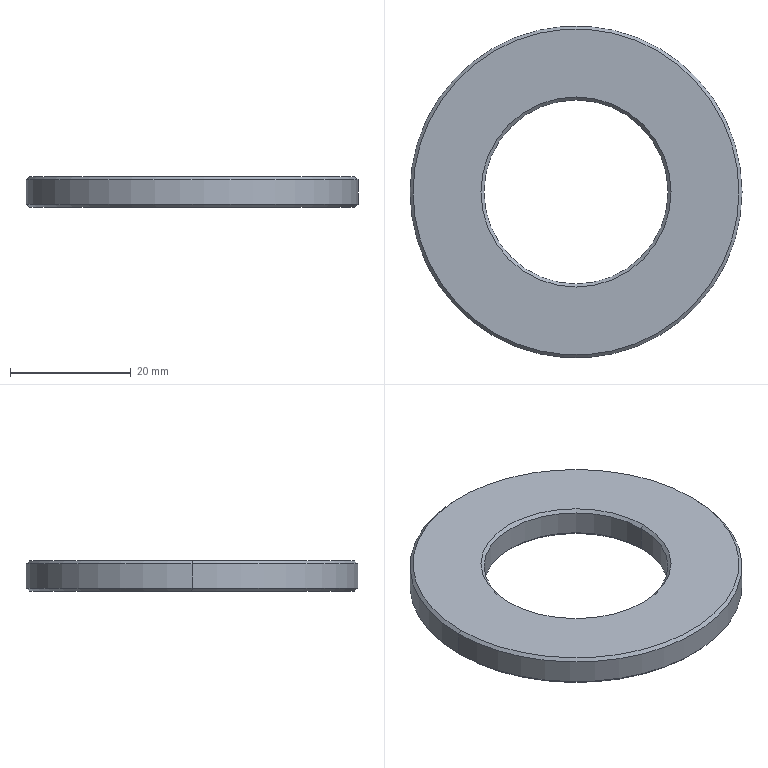Part | STEP file | PN_0001-01-08 Pad | 1 solid | 14 faces | box 55 x 55 x 5 mm | volume 8159 mm3 | cone 8 | cylinder 4 | plane 2 | commonest cylinder face diameters 30.5 x2 55 x2
STEP:
#1=CARTESIAN_POINT('',(27.,0.,5.));
#2=VERTEX_POINT('',#1);
#3=CARTESIAN_POINT('',(-27.,0.,5.));
#4=VERTEX_POINT('',#3);
#5=CARTESIAN_POINT('',(0.,0.,5.));
#6=DIRECTION('',(0.,0.,1.));
#7=DIRECTION('',(1.,0.,0.));
#8=AXIS2_PLACEMENT_3D('',#5,#6,#7);
#9=CIRCLE('',#8,27.);
#10=EDGE_CURVE('',#2,#4,#9,.T.);
#11=ORIENTED_EDGE('',*,*,#10,.F.);
#12=CARTESIAN_POINT('',(27.5,0.,4.5));
#13=VERTEX_POINT('',#12);
#14=CARTESIAN_POINT('',(27.,0.,5.));
#15=DIRECTION('',(0.7071,0.,-0.7071));
#16=VECTOR('',#15,1000.);
#17=LINE('',#14,#16);
#18=EDGE_CURVE('',#2,#13,#17,.T.);
#19=ORIENTED_EDGE('',*,*,#18,.T.);
#20=CARTESIAN_POINT('',(-27.5,0.,4.5));
#21=VERTEX_POINT('',#20);
#22=CARTESIAN_POINT('',(0.,0.,4.5));
#23=DIRECTION('',(0.,0.,-1.));
#24=DIRECTION('',(1.,0.,0.));
#25=AXIS2_PLACEMENT_3D('',#22,#23,#24);
#26=CIRCLE('',#25,27.5);
#27=EDGE_CURVE('',#21,#13,#26,.T.);
#28=ORIENTED_EDGE('',*,*,#27,.F.);
#29=CARTESIAN_POINT('',(-27.,0.,5.));
#30=DIRECTION('',(-0.7071,0.,-0.7071));
#31=VECTOR('',#30,1000.);
#32=LINE('',#29,#31);
#33=EDGE_CURVE('',#4,#21,#32,.T.);
#34=ORIENTED_EDGE('',*,*,#33,.F.);
#35=EDGE_LOOP('',(#11,#19,#28,#34));
#36=FACE_OUTER_BOUND('',#35,.T.);
#37=CARTESIAN_POINT('',(0.,0.,5.));
#38=DIRECTION('',(0.,0.,-1.));
#39=DIRECTION('',(-1.,0.,0.));
#40=AXIS2_PLACEMENT_3D('',#37,#38,#39);
#41=CONICAL_SURFACE('',#40,27.,0.7854);
#42=ADVANCED_FACE('',(#36),#41,.T.);
#43=CARTESIAN_POINT('',(-27.,0.,0.));
#44=VERTEX_POINT('',#43);
#45=CARTESIAN_POINT('',(27.,0.,0.));
#46=VERTEX_POINT('',#45);
#47=CARTESIAN_POINT('',(0.,0.,0.));
#48=DIRECTION('',(0.,0.,-1.));
#49=DIRECTION('',(1.,0.,0.));
#50=AXIS2_PLACEMENT_3D('',#47,#48,#49);
#51=CIRCLE('',#50,27.);
#52=EDGE_CURVE('',#44,#46,#51,.T.);
#53=ORIENTED_EDGE('',*,*,#52,.F.);
#54=CARTESIAN_POINT('',(-27.5,0.,0.5));
#55=VERTEX_POINT('',#54);
#56=CARTESIAN_POINT('',(-27.5,0.,0.5));
#57=DIRECTION('',(-0.7071,0.,0.7071));
#58=VECTOR('',#57,1000.);
#59=LINE('',#56,#58);
#60=EDGE_CURVE('',#44,#55,#59,.T.);
#61=ORIENTED_EDGE('',*,*,#60,.T.);
#62=CARTESIAN_POINT('',(27.5,0.,0.5));
#63=VERTEX_POINT('',#62);
#64=CARTESIAN_POINT('',(0.,0.,0.5));
#65=DIRECTION('',(0.,0.,1.));
#66=DIRECTION('',(1.,0.,0.));
#67=AXIS2_PLACEMENT_3D('',#64,#65,#66);
#68=CIRCLE('',#67,27.5);
#69=EDGE_CURVE('',#63,#55,#68,.T.);
#70=ORIENTED_EDGE('',*,*,#69,.F.);
#71=CARTESIAN_POINT('',(27.5,0.,0.5));
#72=DIRECTION('',(0.7071,0.,0.7071));
#73=VECTOR('',#72,1000.);
#74=LINE('',#71,#73);
#75=EDGE_CURVE('',#46,#63,#74,.T.);
#76=ORIENTED_EDGE('',*,*,#75,.F.);
#77=EDGE_LOOP('',(#53,#61,#70,#76));
#78=FACE_OUTER_BOUND('',#77,.T.);
#79=CARTESIAN_POINT('',(0.,0.,0.5));
#80=DIRECTION('',(0.,0.,1.));
#81=DIRECTION('',(1.,0.,0.));
#82=AXIS2_PLACEMENT_3D('',#79,#80,#81);
#83=CONICAL_SURFACE('',#82,27.5,0.7854);
#84=ADVANCED_FACE('',(#78),#83,.T.);
#85=CARTESIAN_POINT('',(-15.25,0.,4.5));
#86=VERTEX_POINT('',#85);
#87=CARTESIAN_POINT('',(15.25,0.,4.5));
#88=VERTEX_POINT('',#87);
#89=CARTESIAN_POINT('',(0.,0.,4.5));
#90=DIRECTION('',(0.,0.,1.));
#91=DIRECTION('',(1.,0.,0.));
#92=AXIS2_PLACEMENT_3D('',#89,#90,#91);
#93=CIRCLE('',#92,15.25);
#94=EDGE_CURVE('',#86,#88,#93,.T.);
#95=ORIENTED_EDGE('',*,*,#94,.F.);
#96=CARTESIAN_POINT('',(-15.75,0.,5.));
#97=VERTEX_POINT('',#96);
#98=CARTESIAN_POINT('',(-15.25,0.,4.5));
#99=DIRECTION('',(-0.7071,0.,0.7071));
#100=VECTOR('',#99,1000.);
#101=LINE('',#98,#100);
#102=EDGE_CURVE('',#86,#97,#101,.T.);
#103=ORIENTED_EDGE('',*,*,#102,.T.);
#104=CARTESIAN_POINT('',(15.75,0.,5.));
#105=VERTEX_POINT('',#104);
#106=CARTESIAN_POINT('',(0.,0.,5.));
#107=DIRECTION('',(0.,0.,-1.));
#108=DIRECTION('',(1.,0.,0.));
#109=AXIS2_PLACEMENT_3D('',#106,#107,#108);
#110=CIRCLE('',#109,15.75);
#111=EDGE_CURVE('',#105,#97,#110,.T.);
#112=ORIENTED_EDGE('',*,*,#111,.F.);
#113=CARTESIAN_POINT('',(15.25,0.,4.5));
#114=DIRECTION('',(0.7071,0.,0.7071));
#115=VECTOR('',#114,1000.);
#116=LINE('',#113,#115);
#117=EDGE_CURVE('',#88,#105,#116,.T.);
#118=ORIENTED_EDGE('',*,*,#117,.F.);
#119=EDGE_LOOP('',(#95,#103,#112,#118));
#120=FACE_OUTER_BOUND('',#119,.T.);
#121=CARTESIAN_POINT('',(0.,0.,4.5));
#122=DIRECTION('',(0.,0.,1.));
#123=DIRECTION('',(1.,0.,0.));
#124=AXIS2_PLACEMENT_3D('',#121,#122,#123);
#125=CONICAL_SURFACE('',#124,15.25,0.7854);
#126=ADVANCED_FACE('',(#120),#125,.F.);
#127=CARTESIAN_POINT('',(15.25,0.,0.5));
#128=VERTEX_POINT('',#127);
#129=CARTESIAN_POINT('',(-15.25,0.,0.5));
#130=VERTEX_POINT('',#129);
#131=CARTESIAN_POINT('',(0.,0.,0.5));
#132=DIRECTION('',(0.,0.,-1.));
#133=DIRECTION('',(1.,0.,0.));
#134=AXIS2_PLACEMENT_3D('',#131,#132,#133);
#135=CIRCLE('',#134,15.25);
#136=EDGE_CURVE('',#128,#130,#135,.T.);
#137=ORIENTED_EDGE('',*,*,#136,.F.);
#138=CARTESIAN_POINT('',(15.75,0.,0.));
#139=VERTEX_POINT('',#138);
#140=CARTESIAN_POINT('',(15.75,0.,0.));
#141=DIRECTION('',(0.7071,0.,-0.7071));
#142=VECTOR('',#141,1000.);
#143=LINE('',#140,#142);
#144=EDGE_CURVE('',#128,#139,#143,.T.);
#145=ORIENTED_EDGE('',*,*,#144,.T.);
#146=CARTESIAN_POINT('',(-15.75,0.,0.));
#147=VERTEX_POINT('',#146);
#148=CARTESIAN_POINT('',(0.,0.,0.));
#149=DIRECTION('',(0.,0.,1.));
#150=DIRECTION('',(1.,0.,0.));
#151=AXIS2_PLACEMENT_3D('',#148,#149,#150);
#152=CIRCLE('',#151,15.75);
#153=EDGE_CURVE('',#147,#139,#152,.T.);
#154=ORIENTED_EDGE('',*,*,#153,.F.);
#155=CARTESIAN_POINT('',(-15.75,0.,0.));
#156=DIRECTION('',(-0.7071,0.,-0.7071));
#157=VECTOR('',#156,1000.);
#158=LINE('',#155,#157);
#159=EDGE_CURVE('',#130,#147,#158,.T.);
#160=ORIENTED_EDGE('',*,*,#159,.F.);
#161=EDGE_LOOP('',(#137,#145,#154,#160));
#162=FACE_OUTER_BOUND('',#161,.T.);
#163=CARTESIAN_POINT('',(0.,0.,0.));
#164=DIRECTION('',(0.,0.,-1.));
#165=DIRECTION('',(-1.,0.,0.));
#166=AXIS2_PLACEMENT_3D('',#163,#164,#165);
#167=CONICAL_SURFACE('',#166,15.75,0.7854);
#168=ADVANCED_FACE('',(#162),#167,.F.);
#169=ORIENTED_EDGE('',*,*,#94,.T.);
#170=CARTESIAN_POINT('',(15.25,0.,5.));
#171=DIRECTION('',(0.,0.,-1.));
#172=VECTOR('',#171,1000.);
#173=LINE('',#170,#172);
#174=EDGE_CURVE('',#88,#128,#173,.T.);
#175=ORIENTED_EDGE('',*,*,#174,.T.);
#176=ORIENTED_EDGE('',*,*,#136,.T.);
#177=CARTESIAN_POINT('',(-15.25,0.,5.));
#178=DIRECTION('',(0.,0.,-1.));
#179=VECTOR('',#178,1000.);
#180=LINE('',#177,#179);
#181=EDGE_CURVE('',#86,#130,#180,.T.);
#182=ORIENTED_EDGE('',*,*,#181,.F.);
#183=EDGE_LOOP('',(#169,#175,#176,#182));
#184=FACE_OUTER_BOUND('',#183,.T.);
#185=CARTESIAN_POINT('',(0.,0.,5.));
#186=DIRECTION('',(0.,0.,-1.));
#187=DIRECTION('',(-1.,0.,0.));
#188=AXIS2_PLACEMENT_3D('',#185,#186,#187);
#189=CYLINDRICAL_SURFACE('',#188,15.25);
#190=ADVANCED_FACE('',(#184),#189,.F.);
#191=ORIENTED_EDGE('',*,*,#27,.T.);
#192=CARTESIAN_POINT('',(27.5,0.,5.));
#193=DIRECTION('',(0.,0.,-1.));
#194=VECTOR('',#193,1000.);
#195=LINE('',#192,#194);
#196=EDGE_CURVE('',#13,#63,#195,.T.);
#197=ORIENTED_EDGE('',*,*,#196,.T.);
#198=ORIENTED_EDGE('',*,*,#69,.T.);
#199=CARTESIAN_POINT('',(-27.5,0.,5.));
#200=DIRECTION('',(0.,0.,-1.));
#201=VECTOR('',#200,1000.);
#202=LINE('',#199,#201);
#203=EDGE_CURVE('',#21,#55,#202,.T.);
#204=ORIENTED_EDGE('',*,*,#203,.F.);
#205=EDGE_LOOP('',(#191,#197,#198,#204));
#206=FACE_OUTER_BOUND('',#205,.T.);
#207=CARTESIAN_POINT('',(0.,0.,5.));
#208=DIRECTION('',(0.,0.,-1.));
#209=DIRECTION('',(-1.,0.,0.));
#210=AXIS2_PLACEMENT_3D('',#207,#208,#209);
#211=CYLINDRICAL_SURFACE('',#210,27.5);
#212=ADVANCED_FACE('',(#206),#211,.T.);
#213=ORIENTED_EDGE('',*,*,#111,.T.);
#214=CARTESIAN_POINT('',(0.,0.,5.));
#215=DIRECTION('',(0.,0.,-1.));
#216=DIRECTION('',(1.,0.,0.));
#217=AXIS2_PLACEMENT_3D('',#214,#215,#216);
#218=CIRCLE('',#217,15.75);
#219=EDGE_CURVE('',#97,#105,#218,.T.);
#220=ORIENTED_EDGE('',*,*,#219,.T.);
#221=EDGE_LOOP('',(#213,#220));
#222=FACE_BOUND('',#221,.T.);
#223=CARTESIAN_POINT('',(0.,0.,5.));
#224=DIRECTION('',(0.,0.,1.));
#225=DIRECTION('',(1.,0.,0.));
#226=AXIS2_PLACEMENT_3D('',#223,#224,#225);
#227=CIRCLE('',#226,27.);
#228=EDGE_CURVE('',#4,#2,#227,.T.);
#229=ORIENTED_EDGE('',*,*,#228,.T.);
#230=ORIENTED_EDGE('',*,*,#10,.T.);
#231=EDGE_LOOP('',(#229,#230));
#232=FACE_OUTER_BOUND('',#231,.T.);
#233=CARTESIAN_POINT('',(0.,0.,5.));
#234=DIRECTION('',(0.,0.,1.));
#235=DIRECTION('',(1.,0.,0.));
#236=AXIS2_PLACEMENT_3D('',#233,#234,#235);
#237=PLANE('',#236);
#238=ADVANCED_FACE('',(#222,#232),#237,.T.);
#239=ORIENTED_EDGE('',*,*,#153,.T.);
#240=CARTESIAN_POINT('',(0.,0.,0.));
#241=DIRECTION('',(0.,0.,1.));
#242=DIRECTION('',(1.,0.,0.));
#243=AXIS2_PLACEMENT_3D('',#240,#241,#242);
#244=CIRCLE('',#243,15.75);
#245=EDGE_CURVE('',#139,#147,#244,.T.);
#246=ORIENTED_EDGE('',*,*,#245,.T.);
#247=EDGE_LOOP('',(#239,#246));
#248=FACE_BOUND('',#247,.T.);
#249=CARTESIAN_POINT('',(0.,0.,0.));
#250=DIRECTION('',(0.,0.,-1.));
#251=DIRECTION('',(1.,0.,0.));
#252=AXIS2_PLACEMENT_3D('',#249,#250,#251);
#253=CIRCLE('',#252,27.);
#254=EDGE_CURVE('',#46,#44,#253,.T.);
#255=ORIENTED_EDGE('',*,*,#254,.T.);
#256=ORIENTED_EDGE('',*,*,#52,.T.);
#257=EDGE_LOOP('',(#255,#256));
#258=FACE_OUTER_BOUND('',#257,.T.);
#259=CARTESIAN_POINT('',(0.,0.,0.));
#260=DIRECTION('',(0.,0.,1.));
#261=DIRECTION('',(1.,0.,0.));
#262=AXIS2_PLACEMENT_3D('',#259,#260,#261);
#263=PLANE('',#262);
#264=ADVANCED_FACE('',(#248,#258),#263,.F.);
#265=ORIENTED_EDGE('',*,*,#196,.F.);
#266=CARTESIAN_POINT('',(0.,0.,4.5));
#267=DIRECTION('',(0.,0.,-1.));
#268=DIRECTION('',(1.,0.,0.));
#269=AXIS2_PLACEMENT_3D('',#266,#267,#268);
#270=CIRCLE('',#269,27.5);
#271=EDGE_CURVE('',#13,#21,#270,.T.);
#272=ORIENTED_EDGE('',*,*,#271,.T.);
#273=ORIENTED_EDGE('',*,*,#203,.T.);
#274=CARTESIAN_POINT('',(0.,0.,0.5));
#275=DIRECTION('',(0.,0.,1.));
#276=DIRECTION('',(1.,0.,0.));
#277=AXIS2_PLACEMENT_3D('',#274,#275,#276);
#278=CIRCLE('',#277,27.5);
#279=EDGE_CURVE('',#55,#63,#278,.T.);
#280=ORIENTED_EDGE('',*,*,#279,.T.);
#281=EDGE_LOOP('',(#265,#272,#273,#280));
#282=FACE_OUTER_BOUND('',#281,.T.);
#283=CARTESIAN_POINT('',(0.,0.,5.));
#284=DIRECTION('',(0.,0.,-1.));
#285=DIRECTION('',(-1.,0.,0.));
#286=AXIS2_PLACEMENT_3D('',#283,#284,#285);
#287=CYLINDRICAL_SURFACE('',#286,27.5);
#288=ADVANCED_FACE('',(#282),#287,.T.);
#289=ORIENTED_EDGE('',*,*,#174,.F.);
#290=CARTESIAN_POINT('',(0.,0.,4.5));
#291=DIRECTION('',(0.,0.,1.));
#292=DIRECTION('',(1.,0.,0.));
#293=AXIS2_PLACEMENT_3D('',#290,#291,#292);
#294=CIRCLE('',#293,15.25);
#295=EDGE_CURVE('',#88,#86,#294,.T.);
#296=ORIENTED_EDGE('',*,*,#295,.T.);
#297=ORIENTED_EDGE('',*,*,#181,.T.);
#298=CARTESIAN_POINT('',(0.,0.,0.5));
#299=DIRECTION('',(0.,0.,-1.));
#300=DIRECTION('',(1.,0.,0.));
#301=AXIS2_PLACEMENT_3D('',#298,#299,#300);
#302=CIRCLE('',#301,15.25);
#303=EDGE_CURVE('',#130,#128,#302,.T.);
#304=ORIENTED_EDGE('',*,*,#303,.T.);
#305=EDGE_LOOP('',(#289,#296,#297,#304));
#306=FACE_OUTER_BOUND('',#305,.T.);
#307=CARTESIAN_POINT('',(0.,0.,5.));
#308=DIRECTION('',(0.,0.,-1.));
#309=DIRECTION('',(-1.,0.,0.));
#310=AXIS2_PLACEMENT_3D('',#307,#308,#309);
#311=CYLINDRICAL_SURFACE('',#310,15.25);
#312=ADVANCED_FACE('',(#306),#311,.F.);
#313=ORIENTED_EDGE('',*,*,#144,.F.);
#314=ORIENTED_EDGE('',*,*,#303,.F.);
#315=ORIENTED_EDGE('',*,*,#159,.T.);
#316=ORIENTED_EDGE('',*,*,#245,.F.);
#317=EDGE_LOOP('',(#313,#314,#315,#316));
#318=FACE_OUTER_BOUND('',#317,.T.);
#319=CARTESIAN_POINT('',(0.,0.,0.));
#320=DIRECTION('',(0.,0.,-1.));
#321=DIRECTION('',(-1.,0.,0.));
#322=AXIS2_PLACEMENT_3D('',#319,#320,#321);
#323=CONICAL_SURFACE('',#322,15.75,0.7854);
#324=ADVANCED_FACE('',(#318),#323,.F.);
#325=ORIENTED_EDGE('',*,*,#102,.F.);
#326=ORIENTED_EDGE('',*,*,#295,.F.);
#327=ORIENTED_EDGE('',*,*,#117,.T.);
#328=ORIENTED_EDGE('',*,*,#219,.F.);
#329=EDGE_LOOP('',(#325,#326,#327,#328));
#330=FACE_OUTER_BOUND('',#329,.T.);
#331=CARTESIAN_POINT('',(0.,0.,4.5));
#332=DIRECTION('',(0.,0.,1.));
#333=DIRECTION('',(1.,0.,0.));
#334=AXIS2_PLACEMENT_3D('',#331,#332,#333);
#335=CONICAL_SURFACE('',#334,15.25,0.7854);
#336=ADVANCED_FACE('',(#330),#335,.F.);
#337=ORIENTED_EDGE('',*,*,#60,.F.);
#338=ORIENTED_EDGE('',*,*,#254,.F.);
#339=ORIENTED_EDGE('',*,*,#75,.T.);
#340=ORIENTED_EDGE('',*,*,#279,.F.);
#341=EDGE_LOOP('',(#337,#338,#339,#340));
#342=FACE_OUTER_BOUND('',#341,.T.);
#343=CARTESIAN_POINT('',(0.,0.,0.5));
#344=DIRECTION('',(0.,0.,1.));
#345=DIRECTION('',(1.,0.,0.));
#346=AXIS2_PLACEMENT_3D('',#343,#344,#345);
#347=CONICAL_SURFACE('',#346,27.5,0.7854);
#348=ADVANCED_FACE('',(#342),#347,.T.);
#349=ORIENTED_EDGE('',*,*,#18,.F.);
#350=ORIENTED_EDGE('',*,*,#228,.F.);
#351=ORIENTED_EDGE('',*,*,#33,.T.);
#352=ORIENTED_EDGE('',*,*,#271,.F.);
#353=EDGE_LOOP('',(#349,#350,#351,#352));
#354=FACE_OUTER_BOUND('',#353,.T.);
#355=CARTESIAN_POINT('',(0.,0.,5.));
#356=DIRECTION('',(0.,0.,-1.));
#357=DIRECTION('',(-1.,0.,0.));
#358=AXIS2_PLACEMENT_3D('',#355,#356,#357);
#359=CONICAL_SURFACE('',#358,27.,0.7854);
#360=ADVANCED_FACE('',(#354),#359,.T.);
#361=CLOSED_SHELL('',(#42,#84,#126,#168,#190,#212,#238,#264,#288,#312,#324,#336,#348,#360));
#362=MANIFOLD_SOLID_BREP('',#361);
#363=CARTESIAN_POINT('',(0.,0.,0.));
#364=DIRECTION('',(0.,0.,1.));
#365=DIRECTION('',(1.,0.,0.));
#366=AXIS2_PLACEMENT_3D('',#363,#364,#365);
#367=(LENGTH_UNIT()NAMED_UNIT(*)SI_UNIT(.MILLI.,.METRE.));
#368=UNCERTAINTY_MEASURE_WITH_UNIT(LENGTH_MEASURE(0.00001),#367,'','');
#369=(NAMED_UNIT(*)PLANE_ANGLE_UNIT()SI_UNIT($,.RADIAN.));
#370=(NAMED_UNIT(*)SI_UNIT($,.STERADIAN.)SOLID_ANGLE_UNIT());
#371=(GEOMETRIC_REPRESENTATION_CONTEXT(3)GLOBAL_UNCERTAINTY_ASSIGNED_CONTEXT((#368))GLOBAL_UNIT_ASSIGNED_CONTEXT((#367,#369,#370))REPRESENTATION_CONTEXT('',''));
#372=ADVANCED_BREP_SHAPE_REPRESENTATION('',(#362,#366),#371);